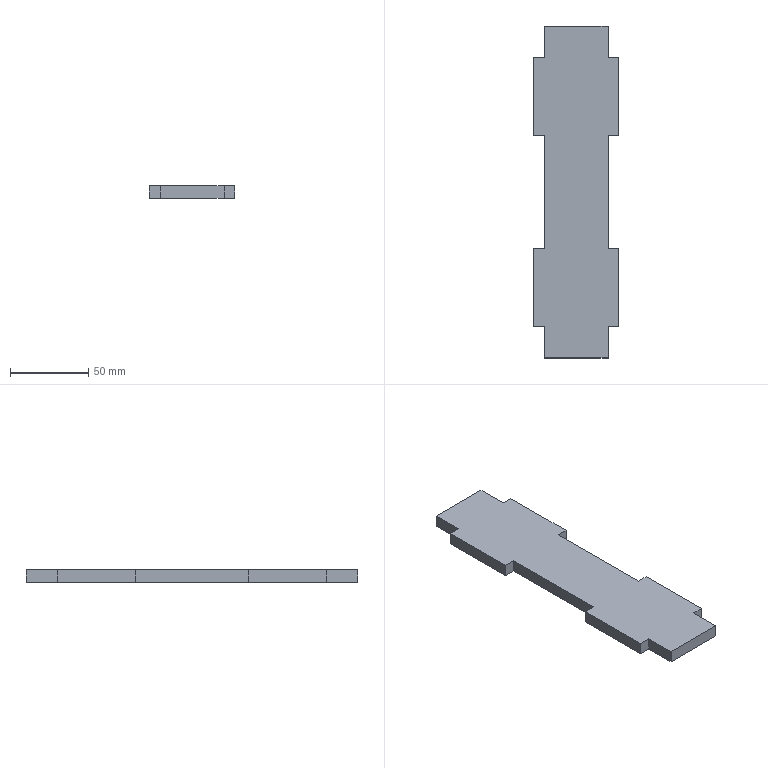Part | SolidWorks | features FlatPattern 1, SMBaseFlange 1, SheetMetal 1 | 1 solid | 22 faces | box 55 x 212.5 x 8 mm | volume 80450 mm3 | plane 22
STEP:
#1=CARTESIAN_POINT('',(-399.005,-131.003,0.));
#2=VERTEX_POINT('',#1);
#3=CARTESIAN_POINT('',(-399.005,-151.003,0.));
#4=VERTEX_POINT('',#3);
#5=CARTESIAN_POINT('',(-399.005,-151.003,0.));
#6=DIRECTION('',(0.,-1.,0.));
#7=VECTOR('',#6,1000.);
#8=LINE('',#5,#7);
#9=EDGE_CURVE('',#2,#4,#8,.T.);
#10=ORIENTED_EDGE('',*,*,#9,.F.);
#11=CARTESIAN_POINT('',(-399.005,-131.003,-8.));
#12=VERTEX_POINT('',#11);
#13=CARTESIAN_POINT('',(-399.005,-131.003,-8.));
#14=DIRECTION('',(0.,0.,1.));
#15=VECTOR('',#14,1000.);
#16=LINE('',#13,#15);
#17=EDGE_CURVE('',#12,#2,#16,.T.);
#18=ORIENTED_EDGE('',*,*,#17,.F.);
#19=CARTESIAN_POINT('',(-399.005,-151.003,-8.));
#20=VERTEX_POINT('',#19);
#21=CARTESIAN_POINT('',(-399.005,-151.003,-8.));
#22=DIRECTION('',(0.,-1.,0.));
#23=VECTOR('',#22,1000.);
#24=LINE('',#21,#23);
#25=EDGE_CURVE('',#12,#20,#24,.T.);
#26=ORIENTED_EDGE('',*,*,#25,.T.);
#27=CARTESIAN_POINT('',(-399.005,-151.003,-8.));
#28=DIRECTION('',(0.,0.,1.));
#29=VECTOR('',#28,1000.);
#30=LINE('',#27,#29);
#31=EDGE_CURVE('',#20,#4,#30,.T.);
#32=ORIENTED_EDGE('',*,*,#31,.T.);
#33=EDGE_LOOP('',(#10,#18,#26,#32));
#34=FACE_OUTER_BOUND('',#33,.T.);
#35=CARTESIAN_POINT('',(-399.005,-151.003,-8.));
#36=DIRECTION('',(-1.,0.,0.));
#37=DIRECTION('',(0.,0.,1.));
#38=AXIS2_PLACEMENT_3D('',#35,#36,#37);
#39=PLANE('',#38);
#40=ADVANCED_FACE('',(#34),#39,.T.);
#41=CARTESIAN_POINT('',(-406.505,-131.003,0.));
#42=VERTEX_POINT('',#41);
#43=CARTESIAN_POINT('',(-399.005,-131.003,0.));
#44=DIRECTION('',(1.,0.,0.));
#45=VECTOR('',#44,1000.);
#46=LINE('',#43,#45);
#47=EDGE_CURVE('',#42,#2,#46,.T.);
#48=ORIENTED_EDGE('',*,*,#47,.F.);
#49=CARTESIAN_POINT('',(-406.505,-131.003,-8.));
#50=VERTEX_POINT('',#49);
#51=CARTESIAN_POINT('',(-406.505,-131.003,-8.));
#52=DIRECTION('',(0.,0.,1.));
#53=VECTOR('',#52,1000.);
#54=LINE('',#51,#53);
#55=EDGE_CURVE('',#50,#42,#54,.T.);
#56=ORIENTED_EDGE('',*,*,#55,.F.);
#57=CARTESIAN_POINT('',(-399.005,-131.003,-8.));
#58=DIRECTION('',(1.,0.,0.));
#59=VECTOR('',#58,1000.);
#60=LINE('',#57,#59);
#61=EDGE_CURVE('',#50,#12,#60,.T.);
#62=ORIENTED_EDGE('',*,*,#61,.T.);
#63=ORIENTED_EDGE('',*,*,#17,.T.);
#64=EDGE_LOOP('',(#48,#56,#62,#63));
#65=FACE_OUTER_BOUND('',#64,.T.);
#66=CARTESIAN_POINT('',(-399.005,-131.003,-8.));
#67=DIRECTION('',(0.,-1.,0.));
#68=DIRECTION('',(0.,0.,-1.));
#69=AXIS2_PLACEMENT_3D('',#66,#67,#68);
#70=PLANE('',#69);
#71=ADVANCED_FACE('',(#65),#70,.T.);
#72=CARTESIAN_POINT('',(-406.505,-81.003,0.));
#73=VERTEX_POINT('',#72);
#74=CARTESIAN_POINT('',(-406.505,-131.003,0.));
#75=DIRECTION('',(0.,-1.,0.));
#76=VECTOR('',#75,1000.);
#77=LINE('',#74,#76);
#78=EDGE_CURVE('',#73,#42,#77,.T.);
#79=ORIENTED_EDGE('',*,*,#78,.F.);
#80=CARTESIAN_POINT('',(-406.505,-81.003,-8.));
#81=VERTEX_POINT('',#80);
#82=CARTESIAN_POINT('',(-406.505,-81.003,-8.));
#83=DIRECTION('',(0.,0.,1.));
#84=VECTOR('',#83,1000.);
#85=LINE('',#82,#84);
#86=EDGE_CURVE('',#81,#73,#85,.T.);
#87=ORIENTED_EDGE('',*,*,#86,.F.);
#88=CARTESIAN_POINT('',(-406.505,-131.003,-8.));
#89=DIRECTION('',(0.,-1.,0.));
#90=VECTOR('',#89,1000.);
#91=LINE('',#88,#90);
#92=EDGE_CURVE('',#81,#50,#91,.T.);
#93=ORIENTED_EDGE('',*,*,#92,.T.);
#94=ORIENTED_EDGE('',*,*,#55,.T.);
#95=EDGE_LOOP('',(#79,#87,#93,#94));
#96=FACE_OUTER_BOUND('',#95,.T.);
#97=CARTESIAN_POINT('',(-406.505,-131.003,-8.));
#98=DIRECTION('',(-1.,0.,0.));
#99=DIRECTION('',(0.,-1.,0.));
#100=AXIS2_PLACEMENT_3D('',#97,#98,#99);
#101=PLANE('',#100);
#102=ADVANCED_FACE('',(#96),#101,.T.);
#103=CARTESIAN_POINT('',(-399.005,-81.003,0.));
#104=VERTEX_POINT('',#103);
#105=CARTESIAN_POINT('',(-406.505,-81.003,0.));
#106=DIRECTION('',(-1.,0.,0.));
#107=VECTOR('',#106,1000.);
#108=LINE('',#105,#107);
#109=EDGE_CURVE('',#104,#73,#108,.T.);
#110=ORIENTED_EDGE('',*,*,#109,.F.);
#111=CARTESIAN_POINT('',(-399.005,-81.003,-8.));
#112=VERTEX_POINT('',#111);
#113=CARTESIAN_POINT('',(-399.005,-81.003,-8.));
#114=DIRECTION('',(0.,0.,1.));
#115=VECTOR('',#114,1000.);
#116=LINE('',#113,#115);
#117=EDGE_CURVE('',#112,#104,#116,.T.);
#118=ORIENTED_EDGE('',*,*,#117,.F.);
#119=CARTESIAN_POINT('',(-406.505,-81.003,-8.));
#120=DIRECTION('',(-1.,0.,0.));
#121=VECTOR('',#120,1000.);
#122=LINE('',#119,#121);
#123=EDGE_CURVE('',#112,#81,#122,.T.);
#124=ORIENTED_EDGE('',*,*,#123,.T.);
#125=ORIENTED_EDGE('',*,*,#86,.T.);
#126=EDGE_LOOP('',(#110,#118,#124,#125));
#127=FACE_OUTER_BOUND('',#126,.T.);
#128=CARTESIAN_POINT('',(-406.505,-81.003,-8.));
#129=DIRECTION('',(0.,1.,0.));
#130=DIRECTION('',(0.,0.,1.));
#131=AXIS2_PLACEMENT_3D('',#128,#129,#130);
#132=PLANE('',#131);
#133=ADVANCED_FACE('',(#127),#132,.T.);
#134=CARTESIAN_POINT('',(-399.005,-8.503,0.));
#135=VERTEX_POINT('',#134);
#136=CARTESIAN_POINT('',(-399.005,-81.003,0.));
#137=DIRECTION('',(0.,-1.,0.));
#138=VECTOR('',#137,1000.);
#139=LINE('',#136,#138);
#140=EDGE_CURVE('',#135,#104,#139,.T.);
#141=ORIENTED_EDGE('',*,*,#140,.F.);
#142=CARTESIAN_POINT('',(-399.005,-8.503,-8.));
#143=VERTEX_POINT('',#142);
#144=CARTESIAN_POINT('',(-399.005,-8.503,-8.));
#145=DIRECTION('',(0.,0.,1.));
#146=VECTOR('',#145,1000.);
#147=LINE('',#144,#146);
#148=EDGE_CURVE('',#143,#135,#147,.T.);
#149=ORIENTED_EDGE('',*,*,#148,.F.);
#150=CARTESIAN_POINT('',(-399.005,-81.003,-8.));
#151=DIRECTION('',(0.,-1.,0.));
#152=VECTOR('',#151,1000.);
#153=LINE('',#150,#152);
#154=EDGE_CURVE('',#143,#112,#153,.T.);
#155=ORIENTED_EDGE('',*,*,#154,.T.);
#156=ORIENTED_EDGE('',*,*,#117,.T.);
#157=EDGE_LOOP('',(#141,#149,#155,#156));
#158=FACE_OUTER_BOUND('',#157,.T.);
#159=CARTESIAN_POINT('',(-399.005,-81.003,-8.));
#160=DIRECTION('',(-1.,0.,0.));
#161=DIRECTION('',(0.,0.,1.));
#162=AXIS2_PLACEMENT_3D('',#159,#160,#161);
#163=PLANE('',#162);
#164=ADVANCED_FACE('',(#158),#163,.T.);
#165=CARTESIAN_POINT('',(-406.505,-8.503,0.));
#166=VERTEX_POINT('',#165);
#167=CARTESIAN_POINT('',(-406.505,-8.503,0.));
#168=DIRECTION('',(1.,0.,0.));
#169=VECTOR('',#168,1000.);
#170=LINE('',#167,#169);
#171=EDGE_CURVE('',#166,#135,#170,.T.);
#172=ORIENTED_EDGE('',*,*,#171,.F.);
#173=CARTESIAN_POINT('',(-406.505,-8.503,-8.));
#174=VERTEX_POINT('',#173);
#175=CARTESIAN_POINT('',(-406.505,-8.503,-8.));
#176=DIRECTION('',(0.,0.,1.));
#177=VECTOR('',#176,1000.);
#178=LINE('',#175,#177);
#179=EDGE_CURVE('',#174,#166,#178,.T.);
#180=ORIENTED_EDGE('',*,*,#179,.F.);
#181=CARTESIAN_POINT('',(-406.505,-8.503,-8.));
#182=DIRECTION('',(1.,0.,0.));
#183=VECTOR('',#182,1000.);
#184=LINE('',#181,#183);
#185=EDGE_CURVE('',#174,#143,#184,.T.);
#186=ORIENTED_EDGE('',*,*,#185,.T.);
#187=ORIENTED_EDGE('',*,*,#148,.T.);
#188=EDGE_LOOP('',(#172,#180,#186,#187));
#189=FACE_OUTER_BOUND('',#188,.T.);
#190=CARTESIAN_POINT('',(-406.505,-8.503,-8.));
#191=DIRECTION('',(0.,-1.,0.));
#192=DIRECTION('',(1.,0.,0.));
#193=AXIS2_PLACEMENT_3D('',#190,#191,#192);
#194=PLANE('',#193);
#195=ADVANCED_FACE('',(#189),#194,.T.);
#196=CARTESIAN_POINT('',(-406.505,41.497,0.));
#197=VERTEX_POINT('',#196);
#198=CARTESIAN_POINT('',(-406.505,41.497,0.));
#199=DIRECTION('',(0.,-1.,0.));
#200=VECTOR('',#199,1000.);
#201=LINE('',#198,#200);
#202=EDGE_CURVE('',#197,#166,#201,.T.);
#203=ORIENTED_EDGE('',*,*,#202,.F.);
#204=CARTESIAN_POINT('',(-406.505,41.497,-8.));
#205=VERTEX_POINT('',#204);
#206=CARTESIAN_POINT('',(-406.505,41.497,-8.));
#207=DIRECTION('',(0.,0.,1.));
#208=VECTOR('',#207,1000.);
#209=LINE('',#206,#208);
#210=EDGE_CURVE('',#205,#197,#209,.T.);
#211=ORIENTED_EDGE('',*,*,#210,.F.);
#212=CARTESIAN_POINT('',(-406.505,41.497,-8.));
#213=DIRECTION('',(0.,-1.,0.));
#214=VECTOR('',#213,1000.);
#215=LINE('',#212,#214);
#216=EDGE_CURVE('',#205,#174,#215,.T.);
#217=ORIENTED_EDGE('',*,*,#216,.T.);
#218=ORIENTED_EDGE('',*,*,#179,.T.);
#219=EDGE_LOOP('',(#203,#211,#217,#218));
#220=FACE_OUTER_BOUND('',#219,.T.);
#221=CARTESIAN_POINT('',(-406.505,41.497,-8.));
#222=DIRECTION('',(-1.,0.,0.));
#223=DIRECTION('',(0.,0.,1.));
#224=AXIS2_PLACEMENT_3D('',#221,#222,#223);
#225=PLANE('',#224);
#226=ADVANCED_FACE('',(#220),#225,.T.);
#227=CARTESIAN_POINT('',(-399.005,41.497,0.));
#228=VERTEX_POINT('',#227);
#229=CARTESIAN_POINT('',(-399.005,41.497,0.));
#230=DIRECTION('',(-1.,0.,0.));
#231=VECTOR('',#230,1000.);
#232=LINE('',#229,#231);
#233=EDGE_CURVE('',#228,#197,#232,.T.);
#234=ORIENTED_EDGE('',*,*,#233,.F.);
#235=CARTESIAN_POINT('',(-399.005,41.497,-8.));
#236=VERTEX_POINT('',#235);
#237=CARTESIAN_POINT('',(-399.005,41.497,-8.));
#238=DIRECTION('',(0.,0.,1.));
#239=VECTOR('',#238,1000.);
#240=LINE('',#237,#239);
#241=EDGE_CURVE('',#236,#228,#240,.T.);
#242=ORIENTED_EDGE('',*,*,#241,.F.);
#243=CARTESIAN_POINT('',(-399.005,41.497,-8.));
#244=DIRECTION('',(-1.,0.,0.));
#245=VECTOR('',#244,1000.);
#246=LINE('',#243,#245);
#247=EDGE_CURVE('',#236,#205,#246,.T.);
#248=ORIENTED_EDGE('',*,*,#247,.T.);
#249=ORIENTED_EDGE('',*,*,#210,.T.);
#250=EDGE_LOOP('',(#234,#242,#248,#249));
#251=FACE_OUTER_BOUND('',#250,.T.);
#252=CARTESIAN_POINT('',(-399.005,41.497,-8.));
#253=DIRECTION('',(0.,1.,0.));
#254=DIRECTION('',(-1.,0.,0.));
#255=AXIS2_PLACEMENT_3D('',#252,#253,#254);
#256=PLANE('',#255);
#257=ADVANCED_FACE('',(#251),#256,.T.);
#258=CARTESIAN_POINT('',(-399.005,61.497,0.));
#259=VERTEX_POINT('',#258);
#260=CARTESIAN_POINT('',(-399.005,41.497,0.));
#261=DIRECTION('',(0.,-1.,0.));
#262=VECTOR('',#261,1000.);
#263=LINE('',#260,#262);
#264=EDGE_CURVE('',#259,#228,#263,.T.);
#265=ORIENTED_EDGE('',*,*,#264,.F.);
#266=CARTESIAN_POINT('',(-399.005,61.497,-8.));
#267=VERTEX_POINT('',#266);
#268=CARTESIAN_POINT('',(-399.005,61.497,-8.));
#269=DIRECTION('',(0.,0.,1.));
#270=VECTOR('',#269,1000.);
#271=LINE('',#268,#270);
#272=EDGE_CURVE('',#267,#259,#271,.T.);
#273=ORIENTED_EDGE('',*,*,#272,.F.);
#274=CARTESIAN_POINT('',(-399.005,41.497,-8.));
#275=DIRECTION('',(0.,-1.,0.));
#276=VECTOR('',#275,1000.);
#277=LINE('',#274,#276);
#278=EDGE_CURVE('',#267,#236,#277,.T.);
#279=ORIENTED_EDGE('',*,*,#278,.T.);
#280=ORIENTED_EDGE('',*,*,#241,.T.);
#281=EDGE_LOOP('',(#265,#273,#279,#280));
#282=FACE_OUTER_BOUND('',#281,.T.);
#283=CARTESIAN_POINT('',(-399.005,41.497,-8.));
#284=DIRECTION('',(-1.,0.,0.));
#285=DIRECTION('',(0.,0.,1.));
#286=AXIS2_PLACEMENT_3D('',#283,#284,#285);
#287=PLANE('',#286);
#288=ADVANCED_FACE('',(#282),#287,.T.);
#289=CARTESIAN_POINT('',(-358.505,61.497,0.));
#290=VERTEX_POINT('',#289);
#291=CARTESIAN_POINT('',(-358.505,61.497,0.));
#292=DIRECTION('',(-1.,0.,0.));
#293=VECTOR('',#292,1000.);
#294=LINE('',#291,#293);
#295=EDGE_CURVE('',#290,#259,#294,.T.);
#296=ORIENTED_EDGE('',*,*,#295,.F.);
#297=CARTESIAN_POINT('',(-358.505,61.497,-8.));
#298=VERTEX_POINT('',#297);
#299=CARTESIAN_POINT('',(-358.505,61.497,-8.));
#300=DIRECTION('',(0.,0.,1.));
#301=VECTOR('',#300,1000.);
#302=LINE('',#299,#301);
#303=EDGE_CURVE('',#298,#290,#302,.T.);
#304=ORIENTED_EDGE('',*,*,#303,.F.);
#305=CARTESIAN_POINT('',(-358.505,61.497,-8.));
#306=DIRECTION('',(-1.,0.,0.));
#307=VECTOR('',#306,1000.);
#308=LINE('',#305,#307);
#309=EDGE_CURVE('',#298,#267,#308,.T.);
#310=ORIENTED_EDGE('',*,*,#309,.T.);
#311=ORIENTED_EDGE('',*,*,#272,.T.);
#312=EDGE_LOOP('',(#296,#304,#310,#311));
#313=FACE_OUTER_BOUND('',#312,.T.);
#314=CARTESIAN_POINT('',(-358.505,61.497,-8.));
#315=DIRECTION('',(0.,1.,0.));
#316=DIRECTION('',(0.,0.,1.));
#317=AXIS2_PLACEMENT_3D('',#314,#315,#316);
#318=PLANE('',#317);
#319=ADVANCED_FACE('',(#313),#318,.T.);
#320=CARTESIAN_POINT('',(-358.505,41.497,0.));
#321=VERTEX_POINT('',#320);
#322=CARTESIAN_POINT('',(-358.505,41.497,0.));
#323=DIRECTION('',(0.,1.,0.));
#324=VECTOR('',#323,1000.);
#325=LINE('',#322,#324);
#326=EDGE_CURVE('',#321,#290,#325,.T.);
#327=ORIENTED_EDGE('',*,*,#326,.F.);
#328=CARTESIAN_POINT('',(-358.505,41.497,-8.));
#329=VERTEX_POINT('',#328);
#330=CARTESIAN_POINT('',(-358.505,41.497,-8.));
#331=DIRECTION('',(0.,0.,1.));
#332=VECTOR('',#331,1000.);
#333=LINE('',#330,#332);
#334=EDGE_CURVE('',#329,#321,#333,.T.);
#335=ORIENTED_EDGE('',*,*,#334,.F.);
#336=CARTESIAN_POINT('',(-358.505,41.497,-8.));
#337=DIRECTION('',(0.,1.,0.));
#338=VECTOR('',#337,1000.);
#339=LINE('',#336,#338);
#340=EDGE_CURVE('',#329,#298,#339,.T.);
#341=ORIENTED_EDGE('',*,*,#340,.T.);
#342=ORIENTED_EDGE('',*,*,#303,.T.);
#343=EDGE_LOOP('',(#327,#335,#341,#342));
#344=FACE_OUTER_BOUND('',#343,.T.);
#345=CARTESIAN_POINT('',(-358.505,41.497,-8.));
#346=DIRECTION('',(1.,0.,0.));
#347=DIRECTION('',(0.,0.,-1.));
#348=AXIS2_PLACEMENT_3D('',#345,#346,#347);
#349=PLANE('',#348);
#350=ADVANCED_FACE('',(#344),#349,.T.);
#351=CARTESIAN_POINT('',(-351.505,41.497,0.));
#352=VERTEX_POINT('',#351);
#353=CARTESIAN_POINT('',(-351.505,41.497,0.));
#354=DIRECTION('',(-1.,0.,0.));
#355=VECTOR('',#354,1000.);
#356=LINE('',#353,#355);
#357=EDGE_CURVE('',#352,#321,#356,.T.);
#358=ORIENTED_EDGE('',*,*,#357,.F.);
#359=CARTESIAN_POINT('',(-351.505,41.497,-8.));
#360=VERTEX_POINT('',#359);
#361=CARTESIAN_POINT('',(-351.505,41.497,-8.));
#362=DIRECTION('',(0.,0.,1.));
#363=VECTOR('',#362,1000.);
#364=LINE('',#361,#363);
#365=EDGE_CURVE('',#360,#352,#364,.T.);
#366=ORIENTED_EDGE('',*,*,#365,.F.);
#367=CARTESIAN_POINT('',(-351.505,41.497,-8.));
#368=DIRECTION('',(-1.,0.,0.));
#369=VECTOR('',#368,1000.);
#370=LINE('',#367,#369);
#371=EDGE_CURVE('',#360,#329,#370,.T.);
#372=ORIENTED_EDGE('',*,*,#371,.T.);
#373=ORIENTED_EDGE('',*,*,#334,.T.);
#374=EDGE_LOOP('',(#358,#366,#372,#373));
#375=FACE_OUTER_BOUND('',#374,.T.);
#376=CARTESIAN_POINT('',(-351.505,41.497,-8.));
#377=DIRECTION('',(0.,1.,0.));
#378=DIRECTION('',(0.,0.,1.));
#379=AXIS2_PLACEMENT_3D('',#376,#377,#378);
#380=PLANE('',#379);
#381=ADVANCED_FACE('',(#375),#380,.T.);
#382=CARTESIAN_POINT('',(-351.505,-8.503,0.));
#383=VERTEX_POINT('',#382);
#384=CARTESIAN_POINT('',(-351.505,-8.503,0.));
#385=DIRECTION('',(0.,1.,0.));
#386=VECTOR('',#385,1000.);
#387=LINE('',#384,#386);
#388=EDGE_CURVE('',#383,#352,#387,.T.);
#389=ORIENTED_EDGE('',*,*,#388,.F.);
#390=CARTESIAN_POINT('',(-351.505,-8.503,-8.));
#391=VERTEX_POINT('',#390);
#392=CARTESIAN_POINT('',(-351.505,-8.503,-8.));
#393=DIRECTION('',(0.,0.,1.));
#394=VECTOR('',#393,1000.);
#395=LINE('',#392,#394);
#396=EDGE_CURVE('',#391,#383,#395,.T.);
#397=ORIENTED_EDGE('',*,*,#396,.F.);
#398=CARTESIAN_POINT('',(-351.505,-8.503,-8.));
#399=DIRECTION('',(0.,1.,0.));
#400=VECTOR('',#399,1000.);
#401=LINE('',#398,#400);
#402=EDGE_CURVE('',#391,#360,#401,.T.);
#403=ORIENTED_EDGE('',*,*,#402,.T.);
#404=ORIENTED_EDGE('',*,*,#365,.T.);
#405=EDGE_LOOP('',(#389,#397,#403,#404));
#406=FACE_OUTER_BOUND('',#405,.T.);
#407=CARTESIAN_POINT('',(-351.505,-8.503,-8.));
#408=DIRECTION('',(1.,0.,0.));
#409=DIRECTION('',(0.,0.,-1.));
#410=AXIS2_PLACEMENT_3D('',#407,#408,#409);
#411=PLANE('',#410);
#412=ADVANCED_FACE('',(#406),#411,.T.);
#413=CARTESIAN_POINT('',(-358.505,-8.503,0.));
#414=VERTEX_POINT('',#413);
#415=CARTESIAN_POINT('',(-358.505,-8.503,0.));
#416=DIRECTION('',(1.,0.,0.));
#417=VECTOR('',#416,1000.);
#418=LINE('',#415,#417);
#419=EDGE_CURVE('',#414,#383,#418,.T.);
#420=ORIENTED_EDGE('',*,*,#419,.F.);
#421=CARTESIAN_POINT('',(-358.505,-8.503,-8.));
#422=VERTEX_POINT('',#421);
#423=CARTESIAN_POINT('',(-358.505,-8.503,-8.));
#424=DIRECTION('',(0.,0.,1.));
#425=VECTOR('',#424,1000.);
#426=LINE('',#423,#425);
#427=EDGE_CURVE('',#422,#414,#426,.T.);
#428=ORIENTED_EDGE('',*,*,#427,.F.);
#429=CARTESIAN_POINT('',(-358.505,-8.503,-8.));
#430=DIRECTION('',(1.,0.,0.));
#431=VECTOR('',#430,1000.);
#432=LINE('',#429,#431);
#433=EDGE_CURVE('',#422,#391,#432,.T.);
#434=ORIENTED_EDGE('',*,*,#433,.T.);
#435=ORIENTED_EDGE('',*,*,#396,.T.);
#436=EDGE_LOOP('',(#420,#428,#434,#435));
#437=FACE_OUTER_BOUND('',#436,.T.);
#438=CARTESIAN_POINT('',(-358.505,-8.503,-8.));
#439=DIRECTION('',(0.,-1.,0.));
#440=DIRECTION('',(0.,0.,-1.));
#441=AXIS2_PLACEMENT_3D('',#438,#439,#440);
#442=PLANE('',#441);
#443=ADVANCED_FACE('',(#437),#442,.T.);
#444=CARTESIAN_POINT('',(-358.505,-81.003,0.));
#445=VERTEX_POINT('',#444);
#446=CARTESIAN_POINT('',(-358.505,-81.003,0.));
#447=DIRECTION('',(0.,1.,0.));
#448=VECTOR('',#447,1000.);
#449=LINE('',#446,#448);
#450=EDGE_CURVE('',#445,#414,#449,.T.);
#451=ORIENTED_EDGE('',*,*,#450,.F.);
#452=CARTESIAN_POINT('',(-358.505,-81.003,-8.));
#453=VERTEX_POINT('',#452);
#454=CARTESIAN_POINT('',(-358.505,-81.003,-8.));
#455=DIRECTION('',(0.,0.,1.));
#456=VECTOR('',#455,1000.);
#457=LINE('',#454,#456);
#458=EDGE_CURVE('',#453,#445,#457,.T.);
#459=ORIENTED_EDGE('',*,*,#458,.F.);
#460=CARTESIAN_POINT('',(-358.505,-81.003,-8.));
#461=DIRECTION('',(0.,1.,0.));
#462=VECTOR('',#461,1000.);
#463=LINE('',#460,#462);
#464=EDGE_CURVE('',#453,#422,#463,.T.);
#465=ORIENTED_EDGE('',*,*,#464,.T.);
#466=ORIENTED_EDGE('',*,*,#427,.T.);
#467=EDGE_LOOP('',(#451,#459,#465,#466));
#468=FACE_OUTER_BOUND('',#467,.T.);
#469=CARTESIAN_POINT('',(-358.505,-81.003,-8.));
#470=DIRECTION('',(1.,0.,0.));
#471=DIRECTION('',(0.,0.,-1.));
#472=AXIS2_PLACEMENT_3D('',#469,#470,#471);
#473=PLANE('',#472);
#474=ADVANCED_FACE('',(#468),#473,.T.);
#475=CARTESIAN_POINT('',(-351.505,-81.003,0.));
#476=VERTEX_POINT('',#475);
#477=CARTESIAN_POINT('',(-351.505,-81.003,0.));
#478=DIRECTION('',(-1.,0.,0.));
#479=VECTOR('',#478,1000.);
#480=LINE('',#477,#479);
#481=EDGE_CURVE('',#476,#445,#480,.T.);
#482=ORIENTED_EDGE('',*,*,#481,.F.);
#483=CARTESIAN_POINT('',(-351.505,-81.003,-8.));
#484=VERTEX_POINT('',#483);
#485=CARTESIAN_POINT('',(-351.505,-81.003,-8.));
#486=DIRECTION('',(0.,0.,1.));
#487=VECTOR('',#486,1000.);
#488=LINE('',#485,#487);
#489=EDGE_CURVE('',#484,#476,#488,.T.);
#490=ORIENTED_EDGE('',*,*,#489,.F.);
#491=CARTESIAN_POINT('',(-351.505,-81.003,-8.));
#492=DIRECTION('',(-1.,0.,0.));
#493=VECTOR('',#492,1000.);
#494=LINE('',#491,#493);
#495=EDGE_CURVE('',#484,#453,#494,.T.);
#496=ORIENTED_EDGE('',*,*,#495,.T.);
#497=ORIENTED_EDGE('',*,*,#458,.T.);
#498=EDGE_LOOP('',(#482,#490,#496,#497));
#499=FACE_OUTER_BOUND('',#498,.T.);
#500=CARTESIAN_POINT('',(-351.505,-81.003,-8.));
#501=DIRECTION('',(0.,1.,0.));
#502=DIRECTION('',(0.,0.,1.));
#503=AXIS2_PLACEMENT_3D('',#500,#501,#502);
#504=PLANE('',#503);
#505=ADVANCED_FACE('',(#499),#504,.T.);
#506=CARTESIAN_POINT('',(-351.505,-131.003,0.));
#507=VERTEX_POINT('',#506);
#508=CARTESIAN_POINT('',(-351.505,-131.003,0.));
#509=DIRECTION('',(0.,1.,0.));
#510=VECTOR('',#509,1000.);
#511=LINE('',#508,#510);
#512=EDGE_CURVE('',#507,#476,#511,.T.);
#513=ORIENTED_EDGE('',*,*,#512,.F.);
#514=CARTESIAN_POINT('',(-351.505,-131.003,-8.));
#515=VERTEX_POINT('',#514);
#516=CARTESIAN_POINT('',(-351.505,-131.003,-8.));
#517=DIRECTION('',(0.,0.,1.));
#518=VECTOR('',#517,1000.);
#519=LINE('',#516,#518);
#520=EDGE_CURVE('',#515,#507,#519,.T.);
#521=ORIENTED_EDGE('',*,*,#520,.F.);
#522=CARTESIAN_POINT('',(-351.505,-131.003,-8.));
#523=DIRECTION('',(0.,1.,0.));
#524=VECTOR('',#523,1000.);
#525=LINE('',#522,#524);
#526=EDGE_CURVE('',#515,#484,#525,.T.);
#527=ORIENTED_EDGE('',*,*,#526,.T.);
#528=ORIENTED_EDGE('',*,*,#489,.T.);
#529=EDGE_LOOP('',(#513,#521,#527,#528));
#530=FACE_OUTER_BOUND('',#529,.T.);
#531=CARTESIAN_POINT('',(-351.505,-131.003,-8.));
#532=DIRECTION('',(1.,0.,0.));
#533=DIRECTION('',(0.,1.,0.));
#534=AXIS2_PLACEMENT_3D('',#531,#532,#533);
#535=PLANE('',#534);
#536=ADVANCED_FACE('',(#530),#535,.T.);
#537=CARTESIAN_POINT('',(-358.505,-131.003,0.));
#538=VERTEX_POINT('',#537);
#539=CARTESIAN_POINT('',(-358.505,-131.003,0.));
#540=DIRECTION('',(1.,0.,0.));
#541=VECTOR('',#540,1000.);
#542=LINE('',#539,#541);
#543=EDGE_CURVE('',#538,#507,#542,.T.);
#544=ORIENTED_EDGE('',*,*,#543,.F.);
#545=CARTESIAN_POINT('',(-358.505,-131.003,-8.));
#546=VERTEX_POINT('',#545);
#547=CARTESIAN_POINT('',(-358.505,-131.003,-8.));
#548=DIRECTION('',(0.,0.,1.));
#549=VECTOR('',#548,1000.);
#550=LINE('',#547,#549);
#551=EDGE_CURVE('',#546,#538,#550,.T.);
#552=ORIENTED_EDGE('',*,*,#551,.F.);
#553=CARTESIAN_POINT('',(-358.505,-131.003,-8.));
#554=DIRECTION('',(1.,0.,0.));
#555=VECTOR('',#554,1000.);
#556=LINE('',#553,#555);
#557=EDGE_CURVE('',#546,#515,#556,.T.);
#558=ORIENTED_EDGE('',*,*,#557,.T.);
#559=ORIENTED_EDGE('',*,*,#520,.T.);
#560=EDGE_LOOP('',(#544,#552,#558,#559));
#561=FACE_OUTER_BOUND('',#560,.T.);
#562=CARTESIAN_POINT('',(-358.505,-131.003,-8.));
#563=DIRECTION('',(0.,-1.,0.));
#564=DIRECTION('',(0.,0.,-1.));
#565=AXIS2_PLACEMENT_3D('',#562,#563,#564);
#566=PLANE('',#565);
#567=ADVANCED_FACE('',(#561),#566,.T.);
#568=CARTESIAN_POINT('',(-358.505,-151.003,0.));
#569=VERTEX_POINT('',#568);
#570=CARTESIAN_POINT('',(-358.505,-151.003,0.));
#571=DIRECTION('',(0.,1.,0.));
#572=VECTOR('',#571,1000.);
#573=LINE('',#570,#572);
#574=EDGE_CURVE('',#569,#538,#573,.T.);
#575=ORIENTED_EDGE('',*,*,#574,.F.);
#576=CARTESIAN_POINT('',(-358.505,-151.003,-8.));
#577=VERTEX_POINT('',#576);
#578=CARTESIAN_POINT('',(-358.505,-151.003,-8.));
#579=DIRECTION('',(0.,0.,1.));
#580=VECTOR('',#579,1000.);
#581=LINE('',#578,#580);
#582=EDGE_CURVE('',#577,#569,#581,.T.);
#583=ORIENTED_EDGE('',*,*,#582,.F.);
#584=CARTESIAN_POINT('',(-358.505,-151.003,-8.));
#585=DIRECTION('',(0.,1.,0.));
#586=VECTOR('',#585,1000.);
#587=LINE('',#584,#586);
#588=EDGE_CURVE('',#577,#546,#587,.T.);
#589=ORIENTED_EDGE('',*,*,#588,.T.);
#590=ORIENTED_EDGE('',*,*,#551,.T.);
#591=EDGE_LOOP('',(#575,#583,#589,#590));
#592=FACE_OUTER_BOUND('',#591,.T.);
#593=CARTESIAN_POINT('',(-358.505,-151.003,-8.));
#594=DIRECTION('',(1.,0.,0.));
#595=DIRECTION('',(0.,0.,-1.));
#596=AXIS2_PLACEMENT_3D('',#593,#594,#595);
#597=PLANE('',#596);
#598=ADVANCED_FACE('',(#592),#597,.T.);
#599=CARTESIAN_POINT('',(-399.005,-151.003,0.));
#600=DIRECTION('',(1.,0.,0.));
#601=VECTOR('',#600,1000.);
#602=LINE('',#599,#601);
#603=EDGE_CURVE('',#4,#569,#602,.T.);
#604=ORIENTED_EDGE('',*,*,#603,.F.);
#605=ORIENTED_EDGE('',*,*,#31,.F.);
#606=CARTESIAN_POINT('',(-399.005,-151.003,-8.));
#607=DIRECTION('',(1.,0.,0.));
#608=VECTOR('',#607,1000.);
#609=LINE('',#606,#608);
#610=EDGE_CURVE('',#20,#577,#609,.T.);
#611=ORIENTED_EDGE('',*,*,#610,.T.);
#612=ORIENTED_EDGE('',*,*,#582,.T.);
#613=EDGE_LOOP('',(#604,#605,#611,#612));
#614=FACE_OUTER_BOUND('',#613,.T.);
#615=CARTESIAN_POINT('',(-399.005,-151.003,-8.));
#616=DIRECTION('',(0.,-1.,0.));
#617=DIRECTION('',(0.,0.,-1.));
#618=AXIS2_PLACEMENT_3D('',#615,#616,#617);
#619=PLANE('',#618);
#620=ADVANCED_FACE('',(#614),#619,.T.);
#621=ORIENTED_EDGE('',*,*,#25,.F.);
#622=ORIENTED_EDGE('',*,*,#61,.F.);
#623=ORIENTED_EDGE('',*,*,#92,.F.);
#624=ORIENTED_EDGE('',*,*,#123,.F.);
#625=ORIENTED_EDGE('',*,*,#154,.F.);
#626=ORIENTED_EDGE('',*,*,#185,.F.);
#627=ORIENTED_EDGE('',*,*,#216,.F.);
#628=ORIENTED_EDGE('',*,*,#247,.F.);
#629=ORIENTED_EDGE('',*,*,#278,.F.);
#630=ORIENTED_EDGE('',*,*,#309,.F.);
#631=ORIENTED_EDGE('',*,*,#340,.F.);
#632=ORIENTED_EDGE('',*,*,#371,.F.);
#633=ORIENTED_EDGE('',*,*,#402,.F.);
#634=ORIENTED_EDGE('',*,*,#433,.F.);
#635=ORIENTED_EDGE('',*,*,#464,.F.);
#636=ORIENTED_EDGE('',*,*,#495,.F.);
#637=ORIENTED_EDGE('',*,*,#526,.F.);
#638=ORIENTED_EDGE('',*,*,#557,.F.);
#639=ORIENTED_EDGE('',*,*,#588,.F.);
#640=ORIENTED_EDGE('',*,*,#610,.F.);
#641=EDGE_LOOP('',(#621,#622,#623,#624,#625,#626,#627,#628,#629,#630,#631,#632,#633,#634,#635,#636,#637,#638,#639,#640));
#642=FACE_OUTER_BOUND('',#641,.T.);
#643=CARTESIAN_POINT('',(0.,0.,-8.));
#644=DIRECTION('',(0.,0.,1.));
#645=DIRECTION('',(1.,0.,0.));
#646=AXIS2_PLACEMENT_3D('',#643,#644,#645);
#647=PLANE('',#646);
#648=ADVANCED_FACE('',(#642),#647,.F.);
#649=ORIENTED_EDGE('',*,*,#9,.T.);
#650=ORIENTED_EDGE('',*,*,#603,.T.);
#651=ORIENTED_EDGE('',*,*,#574,.T.);
#652=ORIENTED_EDGE('',*,*,#543,.T.);
#653=ORIENTED_EDGE('',*,*,#512,.T.);
#654=ORIENTED_EDGE('',*,*,#481,.T.);
#655=ORIENTED_EDGE('',*,*,#450,.T.);
#656=ORIENTED_EDGE('',*,*,#419,.T.);
#657=ORIENTED_EDGE('',*,*,#388,.T.);
#658=ORIENTED_EDGE('',*,*,#357,.T.);
#659=ORIENTED_EDGE('',*,*,#326,.T.);
#660=ORIENTED_EDGE('',*,*,#295,.T.);
#661=ORIENTED_EDGE('',*,*,#264,.T.);
#662=ORIENTED_EDGE('',*,*,#233,.T.);
#663=ORIENTED_EDGE('',*,*,#202,.T.);
#664=ORIENTED_EDGE('',*,*,#171,.T.);
#665=ORIENTED_EDGE('',*,*,#140,.T.);
#666=ORIENTED_EDGE('',*,*,#109,.T.);
#667=ORIENTED_EDGE('',*,*,#78,.T.);
#668=ORIENTED_EDGE('',*,*,#47,.T.);
#669=EDGE_LOOP('',(#649,#650,#651,#652,#653,#654,#655,#656,#657,#658,#659,#660,#661,#662,#663,#664,#665,#666,#667,#668));
#670=FACE_OUTER_BOUND('',#669,.T.);
#671=CARTESIAN_POINT('',(0.,0.,0.));
#672=DIRECTION('',(0.,0.,1.));
#673=DIRECTION('',(1.,0.,0.));
#674=AXIS2_PLACEMENT_3D('',#671,#672,#673);
#675=PLANE('',#674);
#676=ADVANCED_FACE('',(#670),#675,.T.);
#677=CLOSED_SHELL('',(#40,#71,#102,#133,#164,#195,#226,#257,#288,#319,#350,#381,#412,#443,#474,#505,#536,#567,#598,#620,#648,#676));
#678=MANIFOLD_SOLID_BREP('',#677);
#679=CARTESIAN_POINT('',(0.,0.,0.));
#680=DIRECTION('',(0.,0.,1.));
#681=DIRECTION('',(1.,0.,0.));
#682=AXIS2_PLACEMENT_3D('',#679,#680,#681);
#683=(LENGTH_UNIT()NAMED_UNIT(*)SI_UNIT(.MILLI.,.METRE.));
#684=UNCERTAINTY_MEASURE_WITH_UNIT(LENGTH_MEASURE(0.00001),#683,'','');
#685=(NAMED_UNIT(*)PLANE_ANGLE_UNIT()SI_UNIT($,.RADIAN.));
#686=(NAMED_UNIT(*)SI_UNIT($,.STERADIAN.)SOLID_ANGLE_UNIT());
#687=(GEOMETRIC_REPRESENTATION_CONTEXT(3)GLOBAL_UNCERTAINTY_ASSIGNED_CONTEXT((#684))GLOBAL_UNIT_ASSIGNED_CONTEXT((#683,#685,#686))REPRESENTATION_CONTEXT('',''));
#688=ADVANCED_BREP_SHAPE_REPRESENTATION('',(#678,#682),#687);